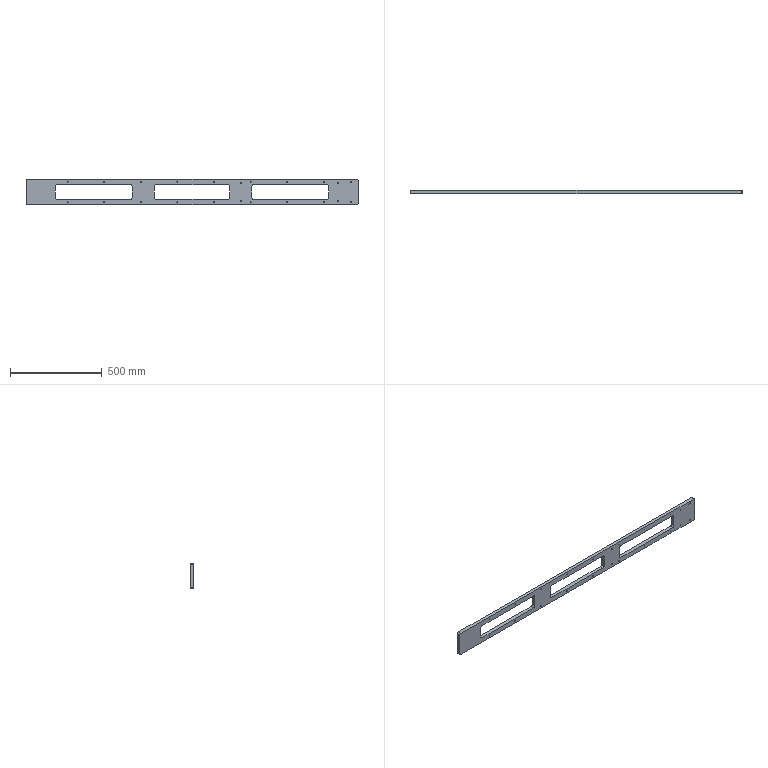Part | SolidWorks | features HoleWzd 3, Chamfer 1, Cut 1, Extrusion 1, Fillet 1 | 1 solid | 98 faces | box 1814 x 20 x 140 mm | volume 3064882 mm3 | cylinder 68 | plane 26 | cone 4 | commonest cylinder face diameters 5 x40 20 x12 6.6 x8 11 x8